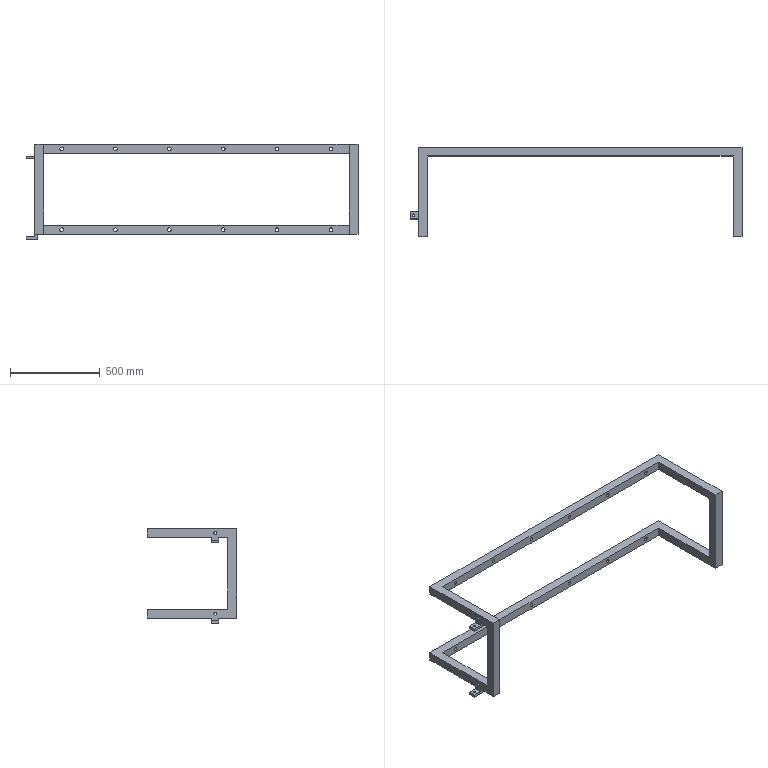Part | SolidWorks | features ICE 11, Extrusion 1, LPattern 1 | 1 solid | 64 faces | box 1848 x 500 x 530 mm | volume 15360816 mm3 | cylinder 36 | plane 28 | commonest cylinder face diameters 20 x24 16 x8 11 x2 15 x2